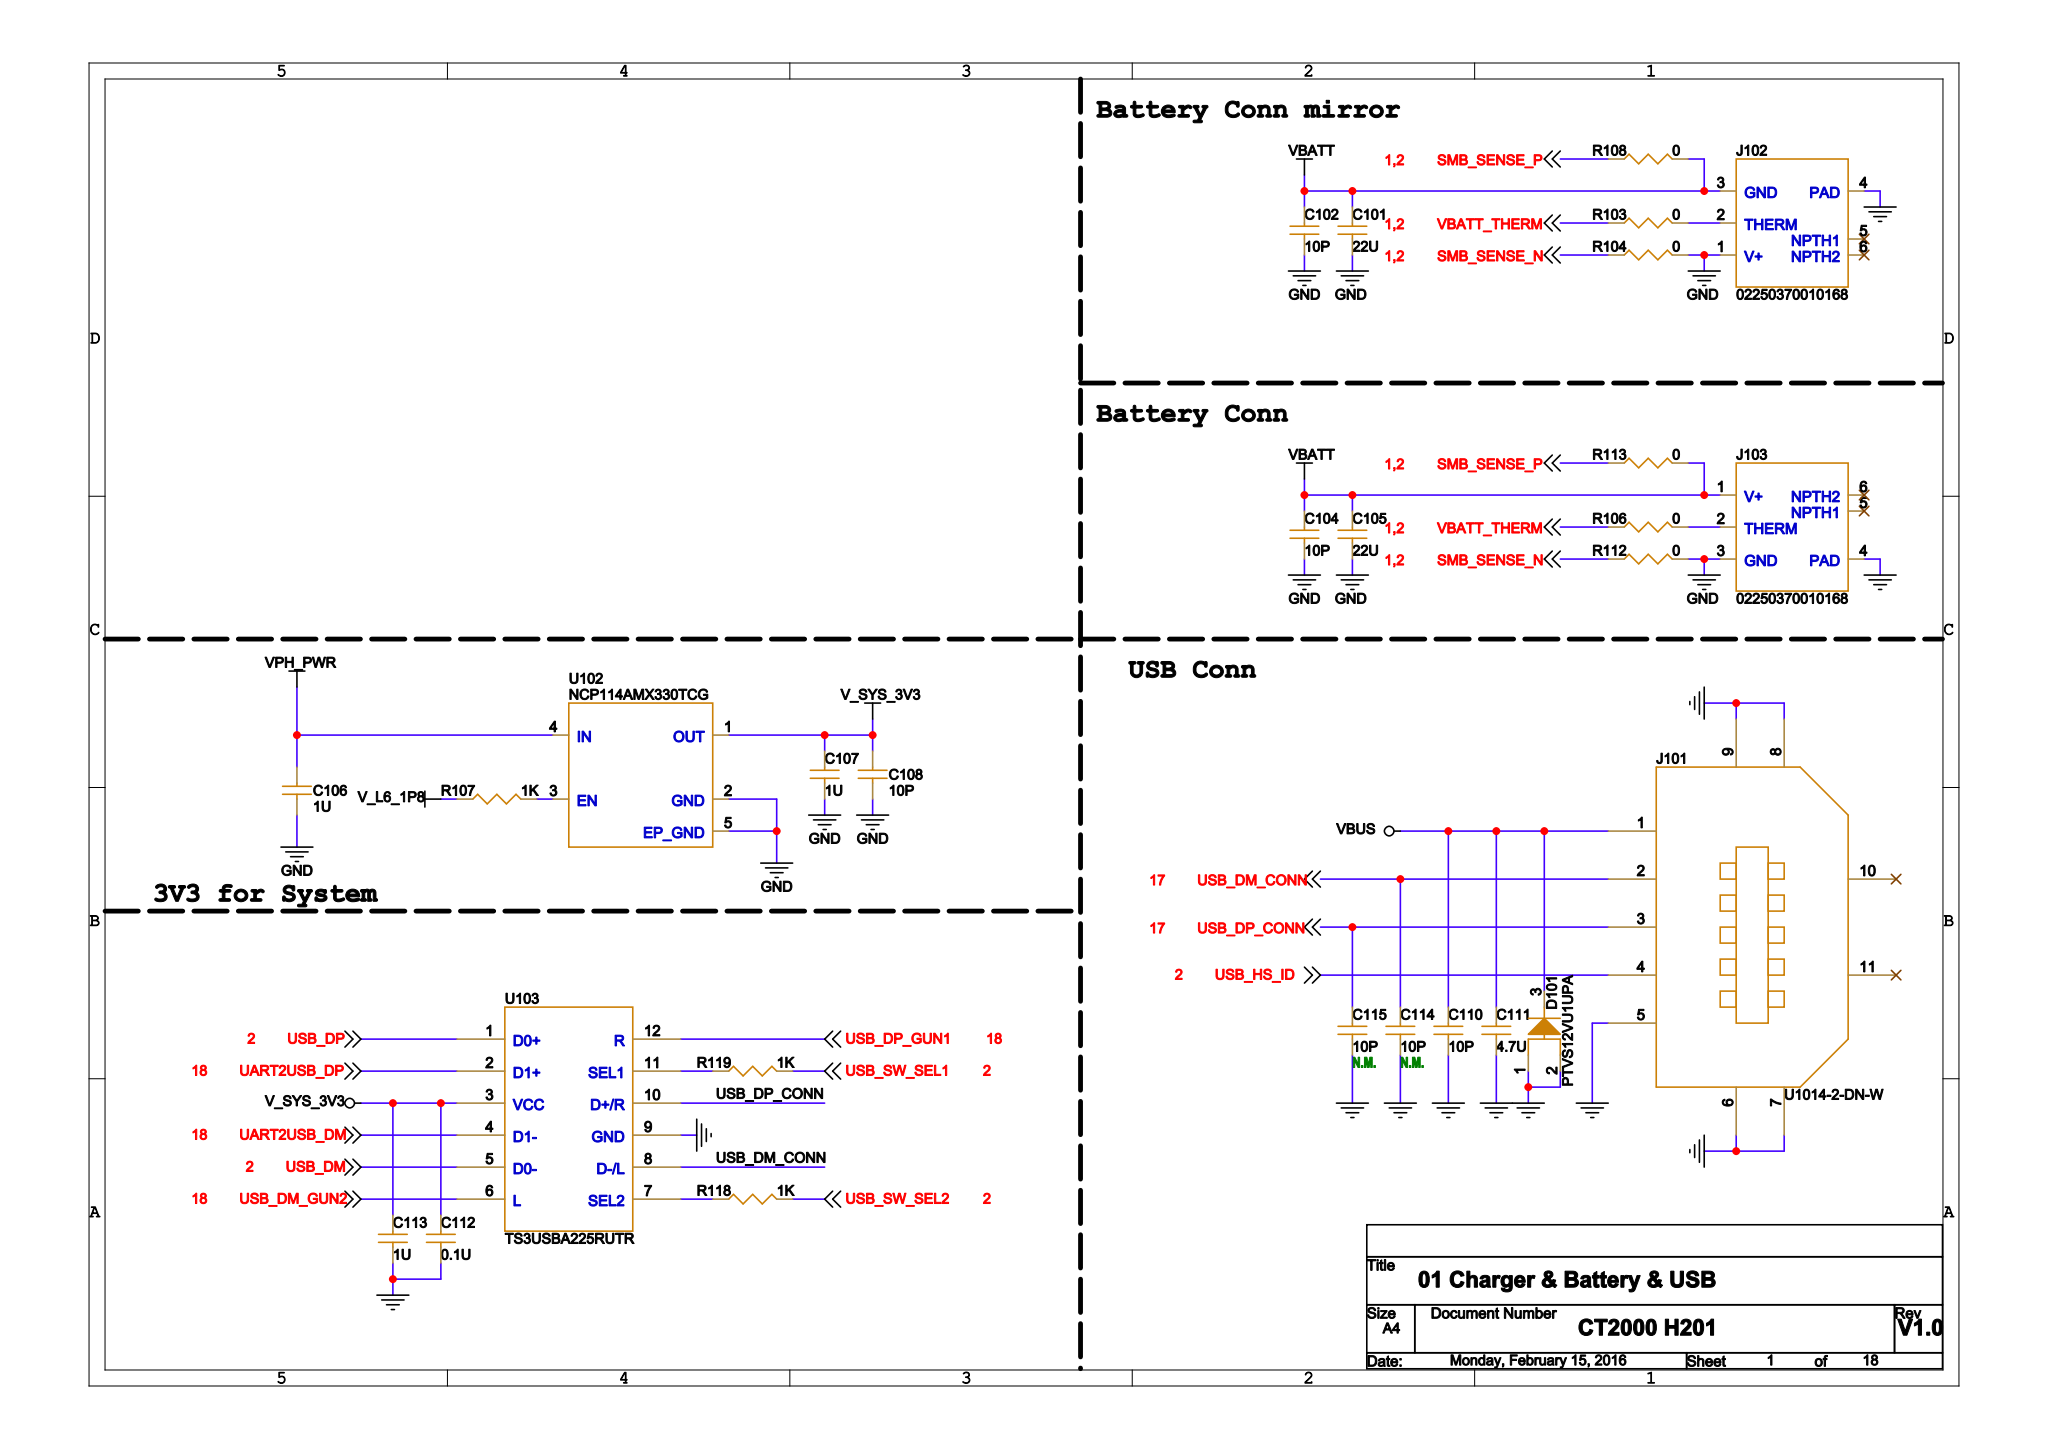Circuit board | Cadence Allegro | 573 parts | 376 nets | one sheet of the schematic
Parts on this sheet (reference | value | footprint):
C101 | 22U | C0805
C102 | 10P | C0402
C104 | 10P | C0402
C105 | 22U | C0805
C106 | 1U | C0402
C107 | 1U | C0402
C108 | 10P | C0402
C110 | 10P | C0402
C111 | 4.7U | C0603
C112 | 0.1U | C0402
C113 | 1U | C0402
C114 | 10P | C0402
C115 | 10P | C0402
D101 | PTVS12VU1UPA | DFN2020-3
J101 | U1014-2-DN-W | USB_U1014-2-DN-W
J102 | 02250370010168 | CON_BAT_02250370010168
J103 | 02250370010168 | CON_BAT_02250370010168
R103 | 0 | R0402
R104 | 0 | R0402
R106 | 0 | R0402
R107 | 1K | R0402
R108 | 0 | R0402
R112 | 0 | R0402
R113 | 0 | R0402
R118 | 1K | R0402
R119 | 1K | R0402
U102 | NCP114AMX330TCG | UDFN4_1X1X0P7_0P65
U103 | TS3USBA225RUTR | UQFN12_2X1P7X0P5_0P4
Nets of these parts (net: part-pin ...):
GND: C101-2 C102-2 C104-2 C105-2 C106-2 C107-2 C108-2 C110-2 C111-2 C112-2 C113-2 C114-2 C115-2 D101-1 D101-2 J101-5 J101-6 J101-7 J101-8 J101-9 J102-1 J102-4 J103-3 J103-4 R104-2 R112-2 U102-2 U102-5 U103-9
UART2USB_DM: U103-4
UART2USB_DP: U103-2
V_SYS_3V3: C107-1 C108-1 C112-1 C113-1 U102-1 U103-3
VBATT: C101-1 C102-1 C104-1 C105-1 J102-3 J103-1 R108-2 R113-2
N52432376: J102-2 R103-2
N52199188: J103-2 R106-2
VPH_PWR: C106-1 U102-4
USB_DP_CONN: C115-1 J101-3 U103-10
USB_DM_CONN: C114-1 J101-2 U103-8
USB_DP: U103-1
USB_DM: U103-5
USB_DM_GUN2: U103-6
USB_DP_GUN1: U103-12
N52583113: R119-1 U103-11
N52583115: R118-1 U103-7
VBUS: C110-1 C111-1 D101-3 J101-1
SMB_SENSE_N: R104-1 R112-1
SMB_SENSE_P: R108-1 R113-1
USB_HS_ID: J101-4
VBATT_THERM: R103-1 R106-1
V_L6_1P8: R107-1
USB_SW_SEL1: R119-2
USB_SW_SEL2: R118-2
N52199208: R107-2 U102-3